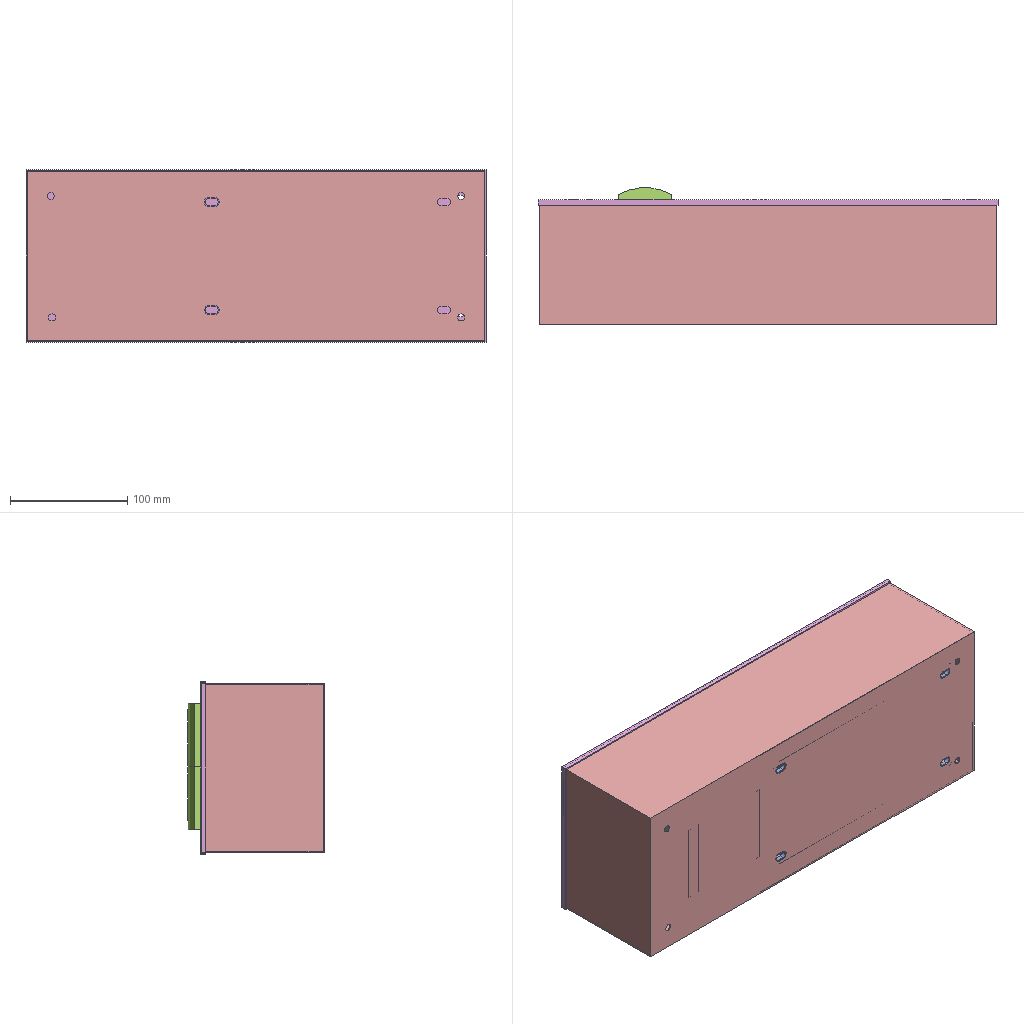Assembly | SolidWorks | 5 different items | 6 placed | box 392 x 116 x 147 mm
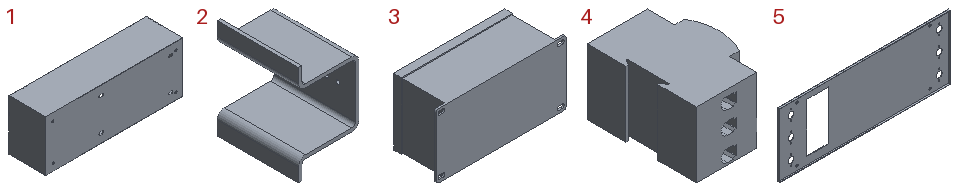Parts list (item | quantity | size | volume | features):
1 | x1 | 390 x 105 x 144.75 mm | 168659 mm3 | features MoveFace 10, ICE 3, Extrusion 1, Fillet 1, HoleWzd 1, Scale 1, Shell 1
2 | x1 | 52 x 70 x 86 mm | 36889 mm3 | features Fillet 2, Extrusion 1, HoleWzd 1, MoveFace 1
3 | x1 | 216 x 86 x 110.411 mm | 1696161 mm3 | features ICE 2, Extrusion 1
4 | x2 | 63.5 x 90 x 54 mm | 247682 mm3 | features ICE 15, MoveFace 7, LPattern 2, Chamfer 1, CombineBodies 1, Extrusion 1, Fillet 1, MirrorPattern 1, PLine 1
5 | x1 | 392.4 x 4.5 x 147.15 mm | 54814 mm3 | features MoveFace 8, ICE 5, Cut 1, Extrusion 1
Mates (type | each side: item.copy, entity, surface, feature):
Coincident | 1.1 face plane Shell1 | 3.1 face plane Boss-Extrude1
Parallel | 1.1 face plane Shell1 | 3.1 face plane Boss-Extrude1
Coincident | 1.1 face plane Boss-Extrude1 | 5.1 face plane Boss-Extrude1 | 2 times
Concentric | 1.1 face cylinder Cut-Extrude1 | 3.1 face cylinder Boss-Extrude1
Coincident | 4.1 face plane Split Line4 | 4.2 face plane LPattern2
Coincident | 4.1 face plane Boss-Extrude1 | 4.2 face plane Boss-Extrude1 | 2 times
Parallel | 1.1 face plane Shell1 | 4.2 face plane Split Line4
DistanceDim | 3.1 face plane Boss-Extrude2 | 4.2 face plane Boss-Extrude1
Coincident | 1.1 face plane Shell1 | 2.1 face plane Boss-Extrude1
Coincident | 4.1 face plane Boss-Extrude1 | 2.1 face plane Boss-Extrude1
DistanceDim | 1.1 face plane Shell1 | 2.1 face plane Boss-Extrude1 | 2 times
DistanceDim | 1.1 face plane Shell1 | 4.1 face plane LPattern2
Concentric | 1.1 face cylinder M4 Tapped Hole1 | 5.1 face cylinder Cut-Extrude1 | 2 times